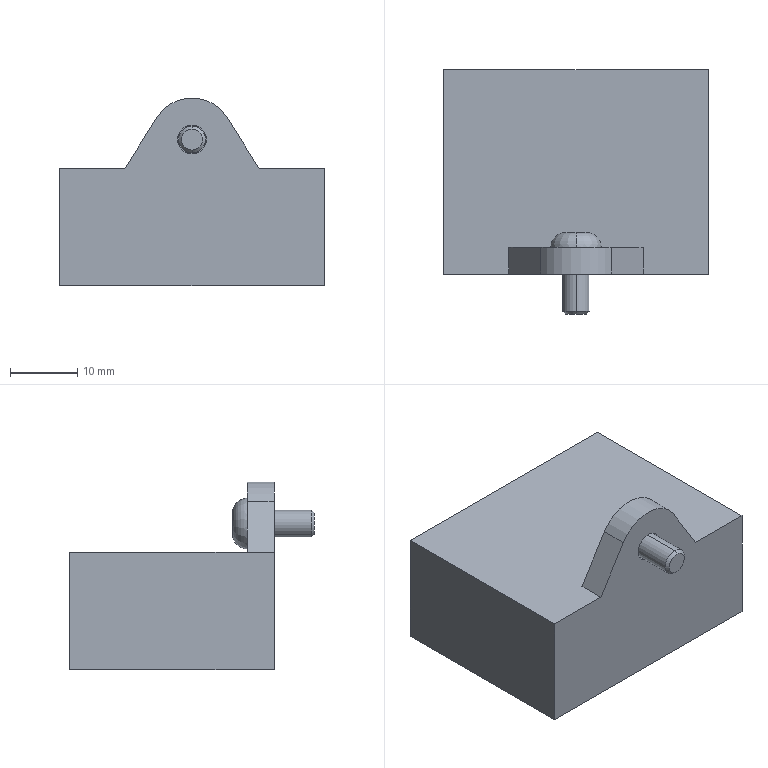Part | STEP file | Guide wheel mechanism revised.sldasm-Part-76 | 1 solid | 28 faces | box 39.5 x 36.5 x 28 mm | volume 21770 mm3 | plane 19 | cylinder 5 | torus 2 | cone 2 | commonest cylinder face diameters 4 x2 4.3 x2 12.4 x1
STEP:
#1=CARTESIAN_POINT('',(0.,4.,8.1));
#2=VERTEX_POINT('',#1);
#3=CARTESIAN_POINT('',(0.,4.,0.5));
#4=VERTEX_POINT('',#3);
#5=CARTESIAN_POINT('',(0.,4.,4.3));
#6=DIRECTION('',(0.,1.,0.));
#7=DIRECTION('',(0.,0.,1.));
#8=AXIS2_PLACEMENT_3D('',#5,#6,#7);
#9=CIRCLE('',#8,3.8);
#10=EDGE_CURVE('',#2,#4,#9,.T.);
#11=ORIENTED_EDGE('',*,*,#10,.T.);
#12=CARTESIAN_POINT('',(0.,6.2,2.7));
#13=VERTEX_POINT('',#12);
#14=CARTESIAN_POINT('',(0.,4.,2.7));
#15=DIRECTION('',(1.,0.,0.));
#16=DIRECTION('',(0.,0.,-1.));
#17=AXIS2_PLACEMENT_3D('',#14,#15,#16);
#18=CIRCLE('',#17,2.2);
#19=EDGE_CURVE('',#4,#13,#18,.T.);
#20=ORIENTED_EDGE('',*,*,#19,.T.);
#21=CARTESIAN_POINT('',(0.,6.2,5.9));
#22=VERTEX_POINT('',#21);
#23=CARTESIAN_POINT('',(0.,6.2,4.3));
#24=DIRECTION('',(0.,1.,0.));
#25=DIRECTION('',(0.,0.,1.));
#26=AXIS2_PLACEMENT_3D('',#23,#24,#25);
#27=CIRCLE('',#26,1.6);
#28=EDGE_CURVE('',#22,#13,#27,.T.);
#29=ORIENTED_EDGE('',*,*,#28,.F.);
#30=CARTESIAN_POINT('',(0.,4.,5.9));
#31=DIRECTION('',(-1.,0.,0.));
#32=DIRECTION('',(0.,0.,1.));
#33=AXIS2_PLACEMENT_3D('',#30,#31,#32);
#34=CIRCLE('',#33,2.2);
#35=EDGE_CURVE('',#2,#22,#34,.T.);
#36=ORIENTED_EDGE('',*,*,#35,.F.);
#37=EDGE_LOOP('',(#11,#20,#29,#36));
#38=FACE_OUTER_BOUND('',#37,.T.);
#39=CARTESIAN_POINT('',(0.,4.,4.3));
#40=DIRECTION('',(0.,1.,0.));
#41=DIRECTION('',(0.,0.,1.));
#42=AXIS2_PLACEMENT_3D('',#39,#40,#41);
#43=TOROIDAL_SURFACE('',#42,1.6,2.2);
#44=ADVANCED_FACE('',(#38),#43,.T.);
#45=CARTESIAN_POINT('',(0.,-5.571,6.3));
#46=VERTEX_POINT('',#45);
#47=CARTESIAN_POINT('',(0.,-5.571,2.3));
#48=VERTEX_POINT('',#47);
#49=CARTESIAN_POINT('',(0.,-5.571,4.3));
#50=DIRECTION('',(0.,1.,0.));
#51=DIRECTION('',(0.,0.,1.));
#52=AXIS2_PLACEMENT_3D('',#49,#50,#51);
#53=CIRCLE('',#52,2.);
#54=EDGE_CURVE('',#46,#48,#53,.T.);
#55=ORIENTED_EDGE('',*,*,#54,.T.);
#56=CARTESIAN_POINT('',(0.,4.,2.3));
#57=VERTEX_POINT('',#56);
#58=CARTESIAN_POINT('',(0.,-6.,2.3));
#59=DIRECTION('',(0.,1.,0.));
#60=VECTOR('',#59,1000.);
#61=LINE('',#58,#60);
#62=EDGE_CURVE('',#48,#57,#61,.T.);
#63=ORIENTED_EDGE('',*,*,#62,.T.);
#64=CARTESIAN_POINT('',(0.,4.,6.3));
#65=VERTEX_POINT('',#64);
#66=CARTESIAN_POINT('',(0.,4.,4.3));
#67=DIRECTION('',(0.,1.,0.));
#68=DIRECTION('',(0.,0.,1.));
#69=AXIS2_PLACEMENT_3D('',#66,#67,#68);
#70=CIRCLE('',#69,2.);
#71=EDGE_CURVE('',#65,#57,#70,.T.);
#72=ORIENTED_EDGE('',*,*,#71,.F.);
#73=CARTESIAN_POINT('',(0.,-6.,6.3));
#74=DIRECTION('',(0.,1.,0.));
#75=VECTOR('',#74,1000.);
#76=LINE('',#73,#75);
#77=EDGE_CURVE('',#46,#65,#76,.T.);
#78=ORIENTED_EDGE('',*,*,#77,.F.);
#79=EDGE_LOOP('',(#55,#63,#72,#78));
#80=FACE_OUTER_BOUND('',#79,.T.);
#81=CARTESIAN_POINT('',(0.,-6.,4.3));
#82=DIRECTION('',(0.,1.,0.));
#83=DIRECTION('',(0.,0.,1.));
#84=AXIS2_PLACEMENT_3D('',#81,#82,#83);
#85=CYLINDRICAL_SURFACE('',#84,2.);
#86=ADVANCED_FACE('',(#80),#85,.T.);
#87=CARTESIAN_POINT('',(0.,-6.,5.87));
#88=VERTEX_POINT('',#87);
#89=CARTESIAN_POINT('',(0.,-6.,2.729));
#90=VERTEX_POINT('',#89);
#91=CARTESIAN_POINT('',(0.,-6.,4.3));
#92=DIRECTION('',(0.,1.,0.));
#93=DIRECTION('',(0.,0.,1.));
#94=AXIS2_PLACEMENT_3D('',#91,#92,#93);
#95=CIRCLE('',#94,1.57);
#96=EDGE_CURVE('',#88,#90,#95,.T.);
#97=ORIENTED_EDGE('',*,*,#96,.T.);
#98=CARTESIAN_POINT('',(0.,-6.,2.73));
#99=DIRECTION('',(0.,0.7071,-0.7071));
#100=VECTOR('',#99,1000.);
#101=LINE('',#98,#100);
#102=EDGE_CURVE('',#90,#48,#101,.T.);
#103=ORIENTED_EDGE('',*,*,#102,.T.);
#104=ORIENTED_EDGE('',*,*,#54,.F.);
#105=CARTESIAN_POINT('',(0.,-6.,5.87));
#106=DIRECTION('',(0.,0.7071,0.7071));
#107=VECTOR('',#106,1000.);
#108=LINE('',#105,#107);
#109=EDGE_CURVE('',#88,#46,#108,.T.);
#110=ORIENTED_EDGE('',*,*,#109,.F.);
#111=EDGE_LOOP('',(#97,#103,#104,#110));
#112=FACE_OUTER_BOUND('',#111,.T.);
#113=CARTESIAN_POINT('',(0.,-6.,4.3));
#114=DIRECTION('',(0.,1.,0.));
#115=DIRECTION('',(0.,0.,1.));
#116=AXIS2_PLACEMENT_3D('',#113,#114,#115);
#117=CONICAL_SURFACE('',#116,1.57,0.7854);
#118=ADVANCED_FACE('',(#112),#117,.T.);
#119=CARTESIAN_POINT('',(0.,0.,2.15));
#120=VERTEX_POINT('',#119);
#121=CARTESIAN_POINT('',(0.,0.,6.45));
#122=VERTEX_POINT('',#121);
#123=CARTESIAN_POINT('',(0.,0.,4.3));
#124=DIRECTION('',(0.,1.,0.));
#125=DIRECTION('',(0.,0.,1.));
#126=AXIS2_PLACEMENT_3D('',#123,#124,#125);
#127=CIRCLE('',#126,2.15);
#128=EDGE_CURVE('',#120,#122,#127,.T.);
#129=ORIENTED_EDGE('',*,*,#128,.F.);
#130=CARTESIAN_POINT('',(0.,4.,2.15));
#131=VERTEX_POINT('',#130);
#132=CARTESIAN_POINT('',(0.,0.,2.15));
#133=DIRECTION('',(0.,1.,0.));
#134=VECTOR('',#133,1000.);
#135=LINE('',#132,#134);
#136=EDGE_CURVE('',#120,#131,#135,.T.);
#137=ORIENTED_EDGE('',*,*,#136,.T.);
#138=CARTESIAN_POINT('',(0.,4.,6.45));
#139=VERTEX_POINT('',#138);
#140=CARTESIAN_POINT('',(0.,4.,4.3));
#141=DIRECTION('',(0.,1.,0.));
#142=DIRECTION('',(0.,0.,1.));
#143=AXIS2_PLACEMENT_3D('',#140,#141,#142);
#144=CIRCLE('',#143,2.15);
#145=EDGE_CURVE('',#131,#139,#144,.T.);
#146=ORIENTED_EDGE('',*,*,#145,.T.);
#147=CARTESIAN_POINT('',(0.,0.,6.45));
#148=DIRECTION('',(0.,1.,0.));
#149=VECTOR('',#148,1000.);
#150=LINE('',#147,#149);
#151=EDGE_CURVE('',#122,#139,#150,.T.);
#152=ORIENTED_EDGE('',*,*,#151,.F.);
#153=EDGE_LOOP('',(#129,#137,#146,#152));
#154=FACE_OUTER_BOUND('',#153,.T.);
#155=CARTESIAN_POINT('',(0.,0.,4.3));
#156=DIRECTION('',(0.,1.,0.));
#157=DIRECTION('',(0.,0.,1.));
#158=AXIS2_PLACEMENT_3D('',#155,#156,#157);
#159=CYLINDRICAL_SURFACE('',#158,2.15);
#160=ADVANCED_FACE('',(#154),#159,.F.);
#161=CARTESIAN_POINT('',(10.,4.,0.));
#162=VERTEX_POINT('',#161);
#163=CARTESIAN_POINT('',(-10.,4.,0.));
#164=VERTEX_POINT('',#163);
#165=CARTESIAN_POINT('',(10.,4.,0.));
#166=DIRECTION('',(-1.,0.,0.));
#167=VECTOR('',#166,1000.);
#168=LINE('',#165,#167);
#169=EDGE_CURVE('',#162,#164,#168,.T.);
#170=ORIENTED_EDGE('',*,*,#169,.T.);
#171=CARTESIAN_POINT('',(-5.257,4.,7.587));
#172=VERTEX_POINT('',#171);
#173=CARTESIAN_POINT('',(-10.,4.,0.));
#174=DIRECTION('',(0.5301,0.,0.8479));
#175=VECTOR('',#174,1000.);
#176=LINE('',#173,#175);
#177=EDGE_CURVE('',#164,#172,#176,.T.);
#178=ORIENTED_EDGE('',*,*,#177,.T.);
#179=CARTESIAN_POINT('',(5.257,4.,7.587));
#180=VERTEX_POINT('',#179);
#181=CARTESIAN_POINT('',(0.,4.,4.3));
#182=DIRECTION('',(0.,1.,0.));
#183=DIRECTION('',(0.,0.,1.));
#184=AXIS2_PLACEMENT_3D('',#181,#182,#183);
#185=CIRCLE('',#184,6.2);
#186=EDGE_CURVE('',#172,#180,#185,.T.);
#187=ORIENTED_EDGE('',*,*,#186,.T.);
#188=CARTESIAN_POINT('',(5.257,4.,7.587));
#189=DIRECTION('',(0.5301,0.,-0.8479));
#190=VECTOR('',#189,1000.);
#191=LINE('',#188,#190);
#192=EDGE_CURVE('',#180,#162,#191,.T.);
#193=ORIENTED_EDGE('',*,*,#192,.T.);
#194=EDGE_LOOP('',(#170,#178,#187,#193));
#195=FACE_OUTER_BOUND('',#194,.T.);
#196=ORIENTED_EDGE('',*,*,#10,.F.);
#197=CARTESIAN_POINT('',(0.,4.,4.3));
#198=DIRECTION('',(0.,1.,0.));
#199=DIRECTION('',(0.,0.,1.));
#200=AXIS2_PLACEMENT_3D('',#197,#198,#199);
#201=CIRCLE('',#200,3.8);
#202=EDGE_CURVE('',#4,#2,#201,.T.);
#203=ORIENTED_EDGE('',*,*,#202,.F.);
#204=EDGE_LOOP('',(#196,#203));
#205=FACE_BOUND('',#204,.T.);
#206=CARTESIAN_POINT('',(0.,4.,4.3));
#207=DIRECTION('',(0.,1.,0.));
#208=DIRECTION('',(0.,0.,1.));
#209=AXIS2_PLACEMENT_3D('',#206,#207,#208);
#210=PLANE('',#209);
#211=ADVANCED_FACE('',(#195,#205),#210,.T.);
#212=CARTESIAN_POINT('',(-19.75,0.,-17.5));
#213=VERTEX_POINT('',#212);
#214=CARTESIAN_POINT('',(-19.75,0.,0.));
#215=VERTEX_POINT('',#214);
#216=CARTESIAN_POINT('',(-19.75,0.,-17.5));
#217=DIRECTION('',(0.,0.,1.));
#218=VECTOR('',#217,1000.);
#219=LINE('',#216,#218);
#220=EDGE_CURVE('',#213,#215,#219,.T.);
#221=ORIENTED_EDGE('',*,*,#220,.F.);
#222=CARTESIAN_POINT('',(19.75,0.,-17.5));
#223=VERTEX_POINT('',#222);
#224=CARTESIAN_POINT('',(19.75,0.,-17.5));
#225=DIRECTION('',(-1.,0.,0.));
#226=VECTOR('',#225,1000.);
#227=LINE('',#224,#226);
#228=EDGE_CURVE('',#223,#213,#227,.T.);
#229=ORIENTED_EDGE('',*,*,#228,.F.);
#230=CARTESIAN_POINT('',(19.75,0.,0.));
#231=VERTEX_POINT('',#230);
#232=CARTESIAN_POINT('',(19.75,0.,0.));
#233=DIRECTION('',(0.,0.,-1.));
#234=VECTOR('',#233,1000.);
#235=LINE('',#232,#234);
#236=EDGE_CURVE('',#231,#223,#235,.T.);
#237=ORIENTED_EDGE('',*,*,#236,.F.);
#238=CARTESIAN_POINT('',(10.,0.,0.));
#239=VERTEX_POINT('',#238);
#240=CARTESIAN_POINT('',(-19.75,0.,0.));
#241=DIRECTION('',(1.,0.,0.));
#242=VECTOR('',#241,1000.);
#243=LINE('',#240,#242);
#244=EDGE_CURVE('',#239,#231,#243,.T.);
#245=ORIENTED_EDGE('',*,*,#244,.F.);
#246=CARTESIAN_POINT('',(5.257,0.,7.587));
#247=VERTEX_POINT('',#246);
#248=CARTESIAN_POINT('',(5.257,0.,7.587));
#249=DIRECTION('',(0.5301,0.,-0.8479));
#250=VECTOR('',#249,1000.);
#251=LINE('',#248,#250);
#252=EDGE_CURVE('',#247,#239,#251,.T.);
#253=ORIENTED_EDGE('',*,*,#252,.F.);
#254=CARTESIAN_POINT('',(-5.257,0.,7.587));
#255=VERTEX_POINT('',#254);
#256=CARTESIAN_POINT('',(0.,0.,4.3));
#257=DIRECTION('',(0.,1.,0.));
#258=DIRECTION('',(0.,0.,1.));
#259=AXIS2_PLACEMENT_3D('',#256,#257,#258);
#260=CIRCLE('',#259,6.2);
#261=EDGE_CURVE('',#255,#247,#260,.T.);
#262=ORIENTED_EDGE('',*,*,#261,.F.);
#263=CARTESIAN_POINT('',(-10.,0.,0.));
#264=VERTEX_POINT('',#263);
#265=CARTESIAN_POINT('',(-10.,0.,0.));
#266=DIRECTION('',(0.5301,0.,0.8479));
#267=VECTOR('',#266,1000.);
#268=LINE('',#265,#267);
#269=EDGE_CURVE('',#264,#255,#268,.T.);
#270=ORIENTED_EDGE('',*,*,#269,.F.);
#271=CARTESIAN_POINT('',(-19.75,0.,0.));
#272=DIRECTION('',(1.,0.,0.));
#273=VECTOR('',#272,1000.);
#274=LINE('',#271,#273);
#275=EDGE_CURVE('',#215,#264,#274,.T.);
#276=ORIENTED_EDGE('',*,*,#275,.F.);
#277=EDGE_LOOP('',(#221,#229,#237,#245,#253,#262,#270,#276));
#278=FACE_OUTER_BOUND('',#277,.T.);
#279=CARTESIAN_POINT('',(0.,0.,4.3));
#280=DIRECTION('',(0.,1.,0.));
#281=DIRECTION('',(0.,0.,1.));
#282=AXIS2_PLACEMENT_3D('',#279,#280,#281);
#283=CIRCLE('',#282,2.15);
#284=EDGE_CURVE('',#122,#120,#283,.T.);
#285=ORIENTED_EDGE('',*,*,#284,.T.);
#286=ORIENTED_EDGE('',*,*,#128,.T.);
#287=EDGE_LOOP('',(#285,#286));
#288=FACE_BOUND('',#287,.T.);
#289=CARTESIAN_POINT('',(0.,0.,0.));
#290=DIRECTION('',(0.,1.,0.));
#291=DIRECTION('',(0.,0.,1.));
#292=AXIS2_PLACEMENT_3D('',#289,#290,#291);
#293=PLANE('',#292);
#294=ADVANCED_FACE('',(#278,#288),#293,.F.);
#295=CARTESIAN_POINT('',(-10.,4.,0.));
#296=DIRECTION('',(0.,-1.,0.));
#297=VECTOR('',#296,1000.);
#298=LINE('',#295,#297);
#299=EDGE_CURVE('',#164,#264,#298,.T.);
#300=ORIENTED_EDGE('',*,*,#299,.F.);
#301=ORIENTED_EDGE('',*,*,#169,.F.);
#302=CARTESIAN_POINT('',(10.,4.,0.));
#303=DIRECTION('',(0.,-1.,0.));
#304=VECTOR('',#303,1000.);
#305=LINE('',#302,#304);
#306=EDGE_CURVE('',#162,#239,#305,.T.);
#307=ORIENTED_EDGE('',*,*,#306,.T.);
#308=ORIENTED_EDGE('',*,*,#244,.T.);
#309=CARTESIAN_POINT('',(19.75,30.5,0.));
#310=VERTEX_POINT('',#309);
#311=CARTESIAN_POINT('',(19.75,30.5,0.));
#312=DIRECTION('',(0.,-1.,0.));
#313=VECTOR('',#312,1000.);
#314=LINE('',#311,#313);
#315=EDGE_CURVE('',#310,#231,#314,.T.);
#316=ORIENTED_EDGE('',*,*,#315,.F.);
#317=CARTESIAN_POINT('',(-19.75,30.5,0.));
#318=VERTEX_POINT('',#317);
#319=CARTESIAN_POINT('',(-19.75,30.5,0.));
#320=DIRECTION('',(1.,0.,0.));
#321=VECTOR('',#320,1000.);
#322=LINE('',#319,#321);
#323=EDGE_CURVE('',#318,#310,#322,.T.);
#324=ORIENTED_EDGE('',*,*,#323,.F.);
#325=CARTESIAN_POINT('',(-19.75,30.5,0.));
#326=DIRECTION('',(0.,-1.,0.));
#327=VECTOR('',#326,1000.);
#328=LINE('',#325,#327);
#329=EDGE_CURVE('',#318,#215,#328,.T.);
#330=ORIENTED_EDGE('',*,*,#329,.T.);
#331=ORIENTED_EDGE('',*,*,#275,.T.);
#332=EDGE_LOOP('',(#300,#301,#307,#308,#316,#324,#330,#331));
#333=FACE_OUTER_BOUND('',#332,.T.);
#334=CARTESIAN_POINT('',(-19.75,30.5,0.));
#335=DIRECTION('',(0.,0.,-1.));
#336=DIRECTION('',(-1.,0.,0.));
#337=AXIS2_PLACEMENT_3D('',#334,#335,#336);
#338=PLANE('',#337);
#339=ADVANCED_FACE('',(#333),#338,.F.);
#340=ORIENTED_EDGE('',*,*,#220,.T.);
#341=ORIENTED_EDGE('',*,*,#329,.F.);
#342=CARTESIAN_POINT('',(-19.75,30.5,-17.5));
#343=VERTEX_POINT('',#342);
#344=CARTESIAN_POINT('',(-19.75,30.5,-17.5));
#345=DIRECTION('',(0.,0.,1.));
#346=VECTOR('',#345,1000.);
#347=LINE('',#344,#346);
#348=EDGE_CURVE('',#343,#318,#347,.T.);
#349=ORIENTED_EDGE('',*,*,#348,.F.);
#350=CARTESIAN_POINT('',(-19.75,30.5,-17.5));
#351=DIRECTION('',(0.,-1.,0.));
#352=VECTOR('',#351,1000.);
#353=LINE('',#350,#352);
#354=EDGE_CURVE('',#343,#213,#353,.T.);
#355=ORIENTED_EDGE('',*,*,#354,.T.);
#356=EDGE_LOOP('',(#340,#341,#349,#355));
#357=FACE_OUTER_BOUND('',#356,.T.);
#358=CARTESIAN_POINT('',(-19.75,30.5,-17.5));
#359=DIRECTION('',(1.,0.,0.));
#360=DIRECTION('',(0.,0.,-1.));
#361=AXIS2_PLACEMENT_3D('',#358,#359,#360);
#362=PLANE('',#361);
#363=ADVANCED_FACE('',(#357),#362,.F.);
#364=ORIENTED_EDGE('',*,*,#236,.T.);
#365=CARTESIAN_POINT('',(19.75,30.5,-17.5));
#366=VERTEX_POINT('',#365);
#367=CARTESIAN_POINT('',(19.75,30.5,-17.5));
#368=DIRECTION('',(0.,-1.,0.));
#369=VECTOR('',#368,1000.);
#370=LINE('',#367,#369);
#371=EDGE_CURVE('',#366,#223,#370,.T.);
#372=ORIENTED_EDGE('',*,*,#371,.F.);
#373=CARTESIAN_POINT('',(19.75,30.5,0.));
#374=DIRECTION('',(0.,0.,-1.));
#375=VECTOR('',#374,1000.);
#376=LINE('',#373,#375);
#377=EDGE_CURVE('',#310,#366,#376,.T.);
#378=ORIENTED_EDGE('',*,*,#377,.F.);
#379=ORIENTED_EDGE('',*,*,#315,.T.);
#380=EDGE_LOOP('',(#364,#372,#378,#379));
#381=FACE_OUTER_BOUND('',#380,.T.);
#382=CARTESIAN_POINT('',(19.75,30.5,0.));
#383=DIRECTION('',(-1.,0.,0.));
#384=DIRECTION('',(0.,0.,1.));
#385=AXIS2_PLACEMENT_3D('',#382,#383,#384);
#386=PLANE('',#385);
#387=ADVANCED_FACE('',(#381),#386,.F.);
#388=ORIENTED_EDGE('',*,*,#228,.T.);
#389=ORIENTED_EDGE('',*,*,#354,.F.);
#390=CARTESIAN_POINT('',(19.75,30.5,-17.5));
#391=DIRECTION('',(-1.,0.,0.));
#392=VECTOR('',#391,1000.);
#393=LINE('',#390,#392);
#394=EDGE_CURVE('',#366,#343,#393,.T.);
#395=ORIENTED_EDGE('',*,*,#394,.F.);
#396=ORIENTED_EDGE('',*,*,#371,.T.);
#397=EDGE_LOOP('',(#388,#389,#395,#396));
#398=FACE_OUTER_BOUND('',#397,.T.);
#399=CARTESIAN_POINT('',(19.75,30.5,-17.5));
#400=DIRECTION('',(0.,0.,1.));
#401=DIRECTION('',(1.,0.,0.));
#402=AXIS2_PLACEMENT_3D('',#399,#400,#401);
#403=PLANE('',#402);
#404=ADVANCED_FACE('',(#398),#403,.F.);
#405=ORIENTED_EDGE('',*,*,#348,.T.);
#406=ORIENTED_EDGE('',*,*,#323,.T.);
#407=ORIENTED_EDGE('',*,*,#377,.T.);
#408=ORIENTED_EDGE('',*,*,#394,.T.);
#409=EDGE_LOOP('',(#405,#406,#407,#408));
#410=FACE_OUTER_BOUND('',#409,.T.);
#411=CARTESIAN_POINT('',(0.,30.5,0.));
#412=DIRECTION('',(0.,1.,0.));
#413=DIRECTION('',(0.,0.,1.));
#414=AXIS2_PLACEMENT_3D('',#411,#412,#413);
#415=PLANE('',#414);
#416=ADVANCED_FACE('',(#410),#415,.T.);
#417=ORIENTED_EDGE('',*,*,#269,.T.);
#418=CARTESIAN_POINT('',(-5.257,4.,7.587));
#419=DIRECTION('',(0.,-1.,0.));
#420=VECTOR('',#419,1000.);
#421=LINE('',#418,#420);
#422=EDGE_CURVE('',#172,#255,#421,.T.);
#423=ORIENTED_EDGE('',*,*,#422,.F.);
#424=ORIENTED_EDGE('',*,*,#177,.F.);
#425=ORIENTED_EDGE('',*,*,#299,.T.);
#426=EDGE_LOOP('',(#417,#423,#424,#425));
#427=FACE_OUTER_BOUND('',#426,.T.);
#428=CARTESIAN_POINT('',(-10.,4.,0.));
#429=DIRECTION('',(0.8479,0.,-0.5301));
#430=DIRECTION('',(-0.5301,0.,-0.8479));
#431=AXIS2_PLACEMENT_3D('',#428,#429,#430);
#432=PLANE('',#431);
#433=ADVANCED_FACE('',(#427),#432,.F.);
#434=ORIENTED_EDGE('',*,*,#261,.T.);
#435=CARTESIAN_POINT('',(5.257,4.,7.587));
#436=DIRECTION('',(0.,-1.,0.));
#437=VECTOR('',#436,1000.);
#438=LINE('',#435,#437);
#439=EDGE_CURVE('',#180,#247,#438,.T.);
#440=ORIENTED_EDGE('',*,*,#439,.F.);
#441=ORIENTED_EDGE('',*,*,#186,.F.);
#442=ORIENTED_EDGE('',*,*,#422,.T.);
#443=EDGE_LOOP('',(#434,#440,#441,#442));
#444=FACE_OUTER_BOUND('',#443,.T.);
#445=CARTESIAN_POINT('',(0.,4.,4.3));
#446=DIRECTION('',(0.,-1.,0.));
#447=DIRECTION('',(0.,0.,-1.));
#448=AXIS2_PLACEMENT_3D('',#445,#446,#447);
#449=CYLINDRICAL_SURFACE('',#448,6.2);
#450=ADVANCED_FACE('',(#444),#449,.T.);
#451=ORIENTED_EDGE('',*,*,#252,.T.);
#452=ORIENTED_EDGE('',*,*,#306,.F.);
#453=ORIENTED_EDGE('',*,*,#192,.F.);
#454=ORIENTED_EDGE('',*,*,#439,.T.);
#455=EDGE_LOOP('',(#451,#452,#453,#454));
#456=FACE_OUTER_BOUND('',#455,.T.);
#457=CARTESIAN_POINT('',(5.257,4.,7.587));
#458=DIRECTION('',(-0.8479,0.,-0.5301));
#459=DIRECTION('',(-0.5301,0.,0.8479));
#460=AXIS2_PLACEMENT_3D('',#457,#458,#459);
#461=PLANE('',#460);
#462=ADVANCED_FACE('',(#456),#461,.F.);
#463=ORIENTED_EDGE('',*,*,#136,.F.);
#464=ORIENTED_EDGE('',*,*,#284,.F.);
#465=ORIENTED_EDGE('',*,*,#151,.T.);
#466=CARTESIAN_POINT('',(0.,4.,4.3));
#467=DIRECTION('',(0.,1.,0.));
#468=DIRECTION('',(0.,0.,1.));
#469=AXIS2_PLACEMENT_3D('',#466,#467,#468);
#470=CIRCLE('',#469,2.15);
#471=EDGE_CURVE('',#139,#131,#470,.T.);
#472=ORIENTED_EDGE('',*,*,#471,.T.);
#473=EDGE_LOOP('',(#463,#464,#465,#472));
#474=FACE_OUTER_BOUND('',#473,.T.);
#475=CARTESIAN_POINT('',(0.,0.,4.3));
#476=DIRECTION('',(0.,1.,0.));
#477=DIRECTION('',(0.,0.,1.));
#478=AXIS2_PLACEMENT_3D('',#475,#476,#477);
#479=CYLINDRICAL_SURFACE('',#478,2.15);
#480=ADVANCED_FACE('',(#474),#479,.F.);
#481=ORIENTED_EDGE('',*,*,#96,.F.);
#482=CARTESIAN_POINT('',(0.,-6.,4.3));
#483=DIRECTION('',(0.,1.,0.));
#484=DIRECTION('',(0.,0.,1.));
#485=AXIS2_PLACEMENT_3D('',#482,#483,#484);
#486=CIRCLE('',#485,1.57);
#487=EDGE_CURVE('',#90,#88,#486,.T.);
#488=ORIENTED_EDGE('',*,*,#487,.F.);
#489=EDGE_LOOP('',(#481,#488));
#490=FACE_OUTER_BOUND('',#489,.T.);
#491=CARTESIAN_POINT('',(1.571,-6.,4.3));
#492=DIRECTION('',(0.,1.,0.));
#493=DIRECTION('',(0.,0.,1.));
#494=AXIS2_PLACEMENT_3D('',#491,#492,#493);
#495=PLANE('',#494);
#496=ADVANCED_FACE('',(#490),#495,.F.);
#497=ORIENTED_EDGE('',*,*,#102,.F.);
#498=ORIENTED_EDGE('',*,*,#487,.T.);
#499=ORIENTED_EDGE('',*,*,#109,.T.);
#500=CARTESIAN_POINT('',(0.,-5.571,4.3));
#501=DIRECTION('',(0.,1.,0.));
#502=DIRECTION('',(0.,0.,1.));
#503=AXIS2_PLACEMENT_3D('',#500,#501,#502);
#504=CIRCLE('',#503,2.);
#505=EDGE_CURVE('',#48,#46,#504,.T.);
#506=ORIENTED_EDGE('',*,*,#505,.F.);
#507=EDGE_LOOP('',(#497,#498,#499,#506));
#508=FACE_OUTER_BOUND('',#507,.T.);
#509=CARTESIAN_POINT('',(0.,-6.,4.3));
#510=DIRECTION('',(0.,1.,0.));
#511=DIRECTION('',(0.,0.,1.));
#512=AXIS2_PLACEMENT_3D('',#509,#510,#511);
#513=CONICAL_SURFACE('',#512,1.57,0.7854);
#514=ADVANCED_FACE('',(#508),#513,.T.);
#515=ORIENTED_EDGE('',*,*,#62,.F.);
#516=ORIENTED_EDGE('',*,*,#505,.T.);
#517=ORIENTED_EDGE('',*,*,#77,.T.);
#518=CARTESIAN_POINT('',(0.,4.,4.3));
#519=DIRECTION('',(0.,1.,0.));
#520=DIRECTION('',(0.,0.,1.));
#521=AXIS2_PLACEMENT_3D('',#518,#519,#520);
#522=CIRCLE('',#521,2.);
#523=EDGE_CURVE('',#57,#65,#522,.T.);
#524=ORIENTED_EDGE('',*,*,#523,.F.);
#525=EDGE_LOOP('',(#515,#516,#517,#524));
#526=FACE_OUTER_BOUND('',#525,.T.);
#527=CARTESIAN_POINT('',(0.,-6.,4.3));
#528=DIRECTION('',(0.,1.,0.));
#529=DIRECTION('',(0.,0.,1.));
#530=AXIS2_PLACEMENT_3D('',#527,#528,#529);
#531=CYLINDRICAL_SURFACE('',#530,2.);
#532=ADVANCED_FACE('',(#526),#531,.T.);
#533=ORIENTED_EDGE('',*,*,#471,.F.);
#534=ORIENTED_EDGE('',*,*,#145,.F.);
#535=EDGE_LOOP('',(#533,#534));
#536=FACE_OUTER_BOUND('',#535,.T.);
#537=ORIENTED_EDGE('',*,*,#71,.T.);
#538=ORIENTED_EDGE('',*,*,#523,.T.);
#539=EDGE_LOOP('',(#537,#538));
#540=FACE_BOUND('',#539,.T.);
#541=CARTESIAN_POINT('',(3.8,4.,4.3));
#542=DIRECTION('',(0.,1.,0.));
#543=DIRECTION('',(0.,0.,1.));
#544=AXIS2_PLACEMENT_3D('',#541,#542,#543);
#545=PLANE('',#544);
#546=ADVANCED_FACE('',(#536,#540),#545,.F.);
#547=CARTESIAN_POINT('',(-1.25,6.2,3.578));
#548=VERTEX_POINT('',#547);
#549=CARTESIAN_POINT('',(-1.25,6.2,5.022));
#550=VERTEX_POINT('',#549);
#551=CARTESIAN_POINT('',(-1.25,6.2,3.578));
#552=DIRECTION('',(0.,0.,1.));
#553=VECTOR('',#552,1000.);
#554=LINE('',#551,#553);
#555=EDGE_CURVE('',#548,#550,#554,.T.);
#556=ORIENTED_EDGE('',*,*,#555,.F.);
#557=CARTESIAN_POINT('',(0.,6.2,2.857));
#558=VERTEX_POINT('',#557);
#559=CARTESIAN_POINT('',(0.,6.2,2.857));
#560=DIRECTION('',(-0.866,0.,0.5));
#561=VECTOR('',#560,1000.);
#562=LINE('',#559,#561);
#563=EDGE_CURVE('',#558,#548,#562,.T.);
#564=ORIENTED_EDGE('',*,*,#563,.F.);
#565=CARTESIAN_POINT('',(1.25,6.2,3.578));
#566=VERTEX_POINT('',#565);
#567=CARTESIAN_POINT('',(1.25,6.2,3.578));
#568=DIRECTION('',(-0.866,0.,-0.5));
#569=VECTOR('',#568,1000.);
#570=LINE('',#567,#569);
#571=EDGE_CURVE('',#566,#558,#570,.T.);
#572=ORIENTED_EDGE('',*,*,#571,.F.);
#573=CARTESIAN_POINT('',(1.25,6.2,5.022));
#574=VERTEX_POINT('',#573);
#575=CARTESIAN_POINT('',(1.25,6.2,5.022));
#576=DIRECTION('',(0.,0.,-1.));
#577=VECTOR('',#576,1000.);
#578=LINE('',#575,#577);
#579=EDGE_CURVE('',#574,#566,#578,.T.);
#580=ORIENTED_EDGE('',*,*,#579,.F.);
#581=CARTESIAN_POINT('',(0.,6.2,5.743));
#582=VERTEX_POINT('',#581);
#583=CARTESIAN_POINT('',(0.,6.2,5.743));
#584=DIRECTION('',(0.866,0.,-0.5));
#585=VECTOR('',#584,1000.);
#586=LINE('',#583,#585);
#587=EDGE_CURVE('',#582,#574,#586,.T.);
#588=ORIENTED_EDGE('',*,*,#587,.F.);
#589=CARTESIAN_POINT('',(-1.25,6.2,5.022));
#590=DIRECTION('',(0.866,0.,0.5));
#591=VECTOR('',#590,1000.);
#592=LINE('',#589,#591);
#593=EDGE_CURVE('',#550,#582,#592,.T.);
#594=ORIENTED_EDGE('',*,*,#593,.F.);
#595=EDGE_LOOP('',(#556,#564,#572,#580,#588,#594));
#596=FACE_BOUND('',#595,.T.);
#597=ORIENTED_EDGE('',*,*,#28,.T.);
#598=CARTESIAN_POINT('',(0.,6.2,4.3));
#599=DIRECTION('',(0.,1.,0.));
#600=DIRECTION('',(0.,0.,1.));
#601=AXIS2_PLACEMENT_3D('',#598,#599,#600);
#602=CIRCLE('',#601,1.6);
#603=EDGE_CURVE('',#13,#22,#602,.T.);
#604=ORIENTED_EDGE('',*,*,#603,.T.);
#605=EDGE_LOOP('',(#597,#604));
#606=FACE_OUTER_BOUND('',#605,.T.);
#607=CARTESIAN_POINT('',(0.,6.2,4.3));
#608=DIRECTION('',(0.,-1.,0.));
#609=DIRECTION('',(0.,0.,-1.));
#610=AXIS2_PLACEMENT_3D('',#607,#608,#609);
#611=PLANE('',#610);
#612=ADVANCED_FACE('',(#596,#606),#611,.F.);
#613=ORIENTED_EDGE('',*,*,#19,.F.);
#614=ORIENTED_EDGE('',*,*,#202,.T.);
#615=ORIENTED_EDGE('',*,*,#35,.T.);
#616=ORIENTED_EDGE('',*,*,#603,.F.);
#617=EDGE_LOOP('',(#613,#614,#615,#616));
#618=FACE_OUTER_BOUND('',#617,.T.);
#619=CARTESIAN_POINT('',(0.,4.,4.3));
#620=DIRECTION('',(0.,1.,0.));
#621=DIRECTION('',(0.,0.,1.));
#622=AXIS2_PLACEMENT_3D('',#619,#620,#621);
#623=TOROIDAL_SURFACE('',#622,1.6,2.2);
#624=ADVANCED_FACE('',(#618),#623,.T.);
#625=ORIENTED_EDGE('',*,*,#563,.T.);
#626=CARTESIAN_POINT('',(-1.25,4.9,3.578));
#627=VERTEX_POINT('',#626);
#628=CARTESIAN_POINT('',(-1.25,4.9,3.578));
#629=DIRECTION('',(0.,1.,0.));
#630=VECTOR('',#629,1000.);
#631=LINE('',#628,#630);
#632=EDGE_CURVE('',#627,#548,#631,.T.);
#633=ORIENTED_EDGE('',*,*,#632,.F.);
#634=CARTESIAN_POINT('',(0.,4.9,2.857));
#635=VERTEX_POINT('',#634);
#636=CARTESIAN_POINT('',(0.,4.9,2.857));
#637=DIRECTION('',(-0.866,0.,0.5));
#638=VECTOR('',#637,1000.);
#639=LINE('',#636,#638);
#640=EDGE_CURVE('',#635,#627,#639,.T.);
#641=ORIENTED_EDGE('',*,*,#640,.F.);
#642=CARTESIAN_POINT('',(0.,4.9,2.857));
#643=DIRECTION('',(0.,1.,0.));
#644=VECTOR('',#643,1000.);
#645=LINE('',#642,#644);
#646=EDGE_CURVE('',#635,#558,#645,.T.);
#647=ORIENTED_EDGE('',*,*,#646,.T.);
#648=EDGE_LOOP('',(#625,#633,#641,#647));
#649=FACE_OUTER_BOUND('',#648,.T.);
#650=CARTESIAN_POINT('',(0.,4.9,2.857));
#651=DIRECTION('',(-0.5,0.,-0.866));
#652=DIRECTION('',(-0.866,0.,0.5));
#653=AXIS2_PLACEMENT_3D('',#650,#651,#652);
#654=PLANE('',#653);
#655=ADVANCED_FACE('',(#649),#654,.F.);
#656=ORIENTED_EDGE('',*,*,#571,.T.);
#657=ORIENTED_EDGE('',*,*,#646,.F.);
#658=CARTESIAN_POINT('',(1.25,4.9,3.578));
#659=VERTEX_POINT('',#658);
#660=CARTESIAN_POINT('',(1.25,4.9,3.578));
#661=DIRECTION('',(-0.866,0.,-0.5));
#662=VECTOR('',#661,1000.);
#663=LINE('',#660,#662);
#664=EDGE_CURVE('',#659,#635,#663,.T.);
#665=ORIENTED_EDGE('',*,*,#664,.F.);
#666=CARTESIAN_POINT('',(1.25,4.9,3.578));
#667=DIRECTION('',(0.,1.,0.));
#668=VECTOR('',#667,1000.);
#669=LINE('',#666,#668);
#670=EDGE_CURVE('',#659,#566,#669,.T.);
#671=ORIENTED_EDGE('',*,*,#670,.T.);
#672=EDGE_LOOP('',(#656,#657,#665,#671));
#673=FACE_OUTER_BOUND('',#672,.T.);
#674=CARTESIAN_POINT('',(1.25,4.9,3.578));
#675=DIRECTION('',(0.5,0.,-0.866));
#676=DIRECTION('',(-0.866,0.,-0.5));
#677=AXIS2_PLACEMENT_3D('',#674,#675,#676);
#678=PLANE('',#677);
#679=ADVANCED_FACE('',(#673),#678,.F.);
#680=ORIENTED_EDGE('',*,*,#579,.T.);
#681=ORIENTED_EDGE('',*,*,#670,.F.);
#682=CARTESIAN_POINT('',(1.25,4.9,5.022));
#683=VERTEX_POINT('',#682);
#684=CARTESIAN_POINT('',(1.25,4.9,5.022));
#685=DIRECTION('',(0.,0.,-1.));
#686=VECTOR('',#685,1000.);
#687=LINE('',#684,#686);
#688=EDGE_CURVE('',#683,#659,#687,.T.);
#689=ORIENTED_EDGE('',*,*,#688,.F.);
#690=CARTESIAN_POINT('',(1.25,4.9,5.022));
#691=DIRECTION('',(0.,1.,0.));
#692=VECTOR('',#691,1000.);
#693=LINE('',#690,#692);
#694=EDGE_CURVE('',#683,#574,#693,.T.);
#695=ORIENTED_EDGE('',*,*,#694,.T.);
#696=EDGE_LOOP('',(#680,#681,#689,#695));
#697=FACE_OUTER_BOUND('',#696,.T.);
#698=CARTESIAN_POINT('',(1.25,4.9,5.022));
#699=DIRECTION('',(1.,0.,0.));
#700=DIRECTION('',(0.,0.,-1.));
#701=AXIS2_PLACEMENT_3D('',#698,#699,#700);
#702=PLANE('',#701);
#703=ADVANCED_FACE('',(#697),#702,.F.);
#704=ORIENTED_EDGE('',*,*,#587,.T.);
#705=ORIENTED_EDGE('',*,*,#694,.F.);
#706=CARTESIAN_POINT('',(0.,4.9,5.743));
#707=VERTEX_POINT('',#706);
#708=CARTESIAN_POINT('',(0.,4.9,5.743));
#709=DIRECTION('',(0.866,0.,-0.5));
#710=VECTOR('',#709,1000.);
#711=LINE('',#708,#710);
#712=EDGE_CURVE('',#707,#683,#711,.T.);
#713=ORIENTED_EDGE('',*,*,#712,.F.);
#714=CARTESIAN_POINT('',(0.,4.9,5.743));
#715=DIRECTION('',(0.,1.,0.));
#716=VECTOR('',#715,1000.);
#717=LINE('',#714,#716);
#718=EDGE_CURVE('',#707,#582,#717,.T.);
#719=ORIENTED_EDGE('',*,*,#718,.T.);
#720=EDGE_LOOP('',(#704,#705,#713,#719));
#721=FACE_OUTER_BOUND('',#720,.T.);
#722=CARTESIAN_POINT('',(0.,4.9,5.743));
#723=DIRECTION('',(0.5,0.,0.866));
#724=DIRECTION('',(0.866,0.,-0.5));
#725=AXIS2_PLACEMENT_3D('',#722,#723,#724);
#726=PLANE('',#725);
#727=ADVANCED_FACE('',(#721),#726,.F.);
#728=ORIENTED_EDGE('',*,*,#593,.T.);
#729=ORIENTED_EDGE('',*,*,#718,.F.);
#730=CARTESIAN_POINT('',(-1.25,4.9,5.022));
#731=VERTEX_POINT('',#730);
#732=CARTESIAN_POINT('',(-1.25,4.9,5.022));
#733=DIRECTION('',(0.866,0.,0.5));
#734=VECTOR('',#733,1000.);
#735=LINE('',#732,#734);
#736=EDGE_CURVE('',#731,#707,#735,.T.);
#737=ORIENTED_EDGE('',*,*,#736,.F.);
#738=CARTESIAN_POINT('',(-1.25,4.9,5.022));
#739=DIRECTION('',(0.,1.,0.));
#740=VECTOR('',#739,1000.);
#741=LINE('',#738,#740);
#742=EDGE_CURVE('',#731,#550,#741,.T.);
#743=ORIENTED_EDGE('',*,*,#742,.T.);
#744=EDGE_LOOP('',(#728,#729,#737,#743));
#745=FACE_OUTER_BOUND('',#744,.T.);
#746=CARTESIAN_POINT('',(-1.25,4.9,5.022));
#747=DIRECTION('',(-0.5,0.,0.866));
#748=DIRECTION('',(0.866,0.,0.5));
#749=AXIS2_PLACEMENT_3D('',#746,#747,#748);
#750=PLANE('',#749);
#751=ADVANCED_FACE('',(#745),#750,.F.);
#752=ORIENTED_EDGE('',*,*,#555,.T.);
#753=ORIENTED_EDGE('',*,*,#742,.F.);
#754=CARTESIAN_POINT('',(-1.25,4.9,3.578));
#755=DIRECTION('',(0.,0.,1.));
#756=VECTOR('',#755,1000.);
#757=LINE('',#754,#756);
#758=EDGE_CURVE('',#627,#731,#757,.T.);
#759=ORIENTED_EDGE('',*,*,#758,.F.);
#760=ORIENTED_EDGE('',*,*,#632,.T.);
#761=EDGE_LOOP('',(#752,#753,#759,#760));
#762=FACE_OUTER_BOUND('',#761,.T.);
#763=CARTESIAN_POINT('',(-1.25,4.9,3.578));
#764=DIRECTION('',(-1.,0.,0.));
#765=DIRECTION('',(0.,0.,1.));
#766=AXIS2_PLACEMENT_3D('',#763,#764,#765);
#767=PLANE('',#766);
#768=ADVANCED_FACE('',(#762),#767,.F.);
#769=ORIENTED_EDGE('',*,*,#640,.T.);
#770=ORIENTED_EDGE('',*,*,#758,.T.);
#771=ORIENTED_EDGE('',*,*,#736,.T.);
#772=ORIENTED_EDGE('',*,*,#712,.T.);
#773=ORIENTED_EDGE('',*,*,#688,.T.);
#774=ORIENTED_EDGE('',*,*,#664,.T.);
#775=EDGE_LOOP('',(#769,#770,#771,#772,#773,#774));
#776=FACE_OUTER_BOUND('',#775,.T.);
#777=CARTESIAN_POINT('',(0.,4.9,0.));
#778=DIRECTION('',(0.,1.,0.));
#779=DIRECTION('',(0.,0.,1.));
#780=AXIS2_PLACEMENT_3D('',#777,#778,#779);
#781=PLANE('',#780);
#782=ADVANCED_FACE('',(#776),#781,.T.);
#783=CLOSED_SHELL('',(#44,#86,#118,#160,#211,#294,#339,#363,#387,#404,#416,#433,#450,#462,#480,#496,#514,#532,#546,#612,#624,#655,#679,#703,#727,#751,#768,#782));
#784=MANIFOLD_SOLID_BREP('',#783);
#785=CARTESIAN_POINT('',(0.,0.,0.));
#786=DIRECTION('',(0.,0.,1.));
#787=DIRECTION('',(1.,0.,0.));
#788=AXIS2_PLACEMENT_3D('',#785,#786,#787);
#789=(LENGTH_UNIT()NAMED_UNIT(*)SI_UNIT(.MILLI.,.METRE.));
#790=UNCERTAINTY_MEASURE_WITH_UNIT(LENGTH_MEASURE(0.00001),#789,'','');
#791=(NAMED_UNIT(*)PLANE_ANGLE_UNIT()SI_UNIT($,.RADIAN.));
#792=(NAMED_UNIT(*)SI_UNIT($,.STERADIAN.)SOLID_ANGLE_UNIT());
#793=(GEOMETRIC_REPRESENTATION_CONTEXT(3)GLOBAL_UNCERTAINTY_ASSIGNED_CONTEXT((#790))GLOBAL_UNIT_ASSIGNED_CONTEXT((#789,#791,#792))REPRESENTATION_CONTEXT('',''));
#794=ADVANCED_BREP_SHAPE_REPRESENTATION('',(#784,#788),#793);